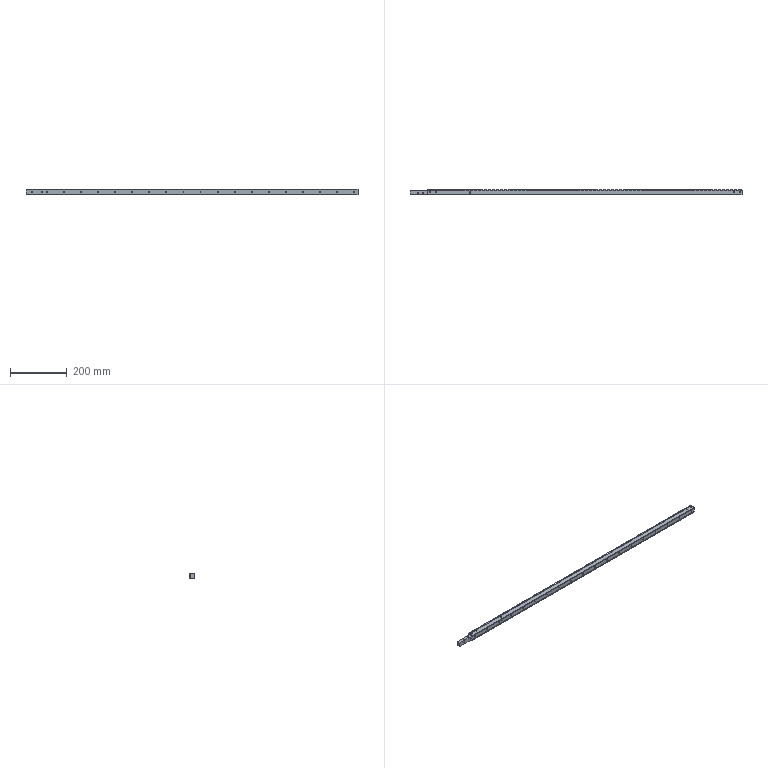Part | STEP file | X77-04011 | 1 solid | 1058 faces | box 1170 x 20 x 20 mm | volume 371955 mm3 | plane 954 | cylinder 58 | cone 46 | commonest cylinder face diameters 3.3 x46 4.2 x8 5 x2 11 x2